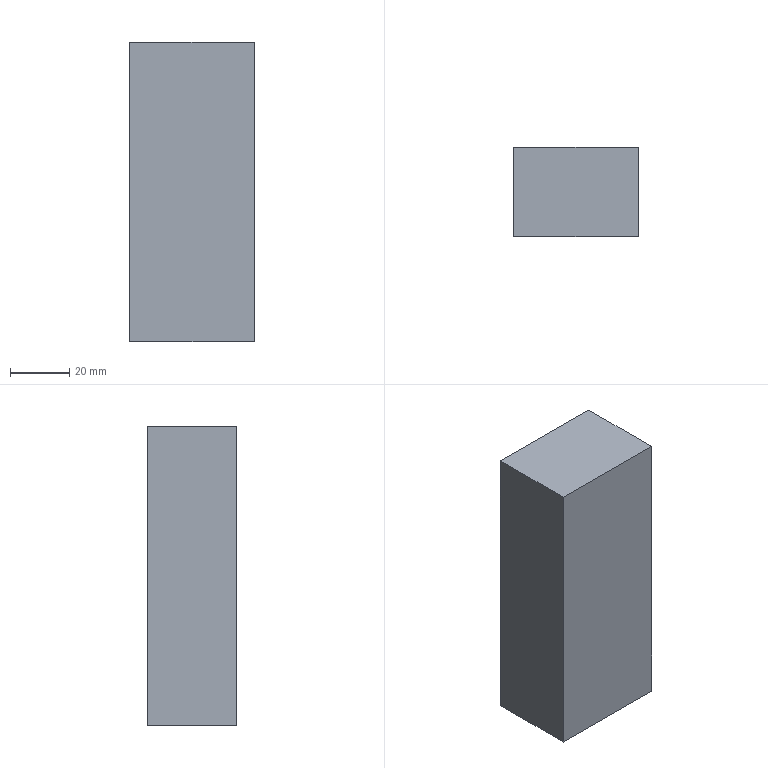Part | NX | features M5 螺纹孔1 2 | 1 solid | 6 faces | box 42 x 30 x 101 mm | volume 127260 mm3 | plane 6
STEP:
#1=CARTESIAN_POINT('',(-21.,201.666,187.866));
#2=VERTEX_POINT('',#1);
#3=CARTESIAN_POINT('',(-21.,201.666,86.866));
#4=VERTEX_POINT('',#3);
#5=CARTESIAN_POINT('',(-21.,201.666,116.575));
#6=DIRECTION('',(-0.000000012,0.,-1.));
#7=VECTOR('',#6,1000.);
#8=LINE('',#5,#7);
#9=EDGE_CURVE('',#2,#4,#8,.T.);
#10=ORIENTED_EDGE('',*,*,#9,.T.);
#11=CARTESIAN_POINT('',(-21.,171.666,86.866));
#12=VERTEX_POINT('',#11);
#13=CARTESIAN_POINT('',(-21.,137.875,86.866));
#14=DIRECTION('',(0.000000003,-1.,0.));
#15=VECTOR('',#14,1000.);
#16=LINE('',#13,#15);
#17=EDGE_CURVE('',#4,#12,#16,.T.);
#18=ORIENTED_EDGE('',*,*,#17,.T.);
#19=CARTESIAN_POINT('',(-21.,171.666,187.866));
#20=VERTEX_POINT('',#19);
#21=CARTESIAN_POINT('',(-21.,171.666,116.575));
#22=DIRECTION('',(-0.000000012,0.,-1.));
#23=VECTOR('',#22,1000.);
#24=LINE('',#21,#23);
#25=EDGE_CURVE('',#20,#12,#24,.T.);
#26=ORIENTED_EDGE('',*,*,#25,.F.);
#27=CARTESIAN_POINT('',(-21.,201.966,187.866));
#28=DIRECTION('',(0.000000003,-1.,0.));
#29=VECTOR('',#28,1000.);
#30=LINE('',#27,#29);
#31=EDGE_CURVE('',#2,#20,#30,.T.);
#32=ORIENTED_EDGE('',*,*,#31,.F.);
#33=EDGE_LOOP('',(#10,#18,#26,#32));
#34=FACE_BOUND('',#33,.T.);
#35=CARTESIAN_POINT('',(-21.,137.875,116.575));
#36=DIRECTION('',(1.,0.000000003,-0.000000012));
#37=DIRECTION('',(0.000000012,0.,1.));
#38=AXIS2_PLACEMENT_3D('',#35,#36,#37);
#39=PLANE('',#38);
#40=ADVANCED_FACE('',(#34),#39,.F.);
#41=CARTESIAN_POINT('',(21.,201.666,86.866));
#42=VERTEX_POINT('',#41);
#43=CARTESIAN_POINT('',(-25.,201.666,86.866));
#44=DIRECTION('',(1.,0.,-0.000000009));
#45=VECTOR('',#44,1000.);
#46=LINE('',#43,#45);
#47=EDGE_CURVE('',#4,#42,#46,.T.);
#48=ORIENTED_EDGE('',*,*,#47,.T.);
#49=CARTESIAN_POINT('',(21.,171.666,86.866));
#50=VERTEX_POINT('',#49);
#51=CARTESIAN_POINT('',(21.,130.666,86.866));
#52=DIRECTION('',(0.,-1.,0.));
#53=VECTOR('',#52,1000.);
#54=LINE('',#51,#53);
#55=EDGE_CURVE('',#42,#50,#54,.T.);
#56=ORIENTED_EDGE('',*,*,#55,.T.);
#57=CARTESIAN_POINT('',(-25.,171.666,86.866));
#58=DIRECTION('',(1.,0.,-0.000000009));
#59=VECTOR('',#58,1000.);
#60=LINE('',#57,#59);
#61=EDGE_CURVE('',#12,#50,#60,.T.);
#62=ORIENTED_EDGE('',*,*,#61,.F.);
#63=ORIENTED_EDGE('',*,*,#17,.F.);
#64=EDGE_LOOP('',(#48,#56,#62,#63));
#65=FACE_BOUND('',#64,.T.);
#66=CARTESIAN_POINT('',(-25.,130.666,86.866));
#67=DIRECTION('',(0.000000009,0.,1.));
#68=DIRECTION('',(0.,1.,0.));
#69=AXIS2_PLACEMENT_3D('',#66,#67,#68);
#70=PLANE('',#69);
#71=ADVANCED_FACE('',(#65),#70,.F.);
#72=CARTESIAN_POINT('',(21.,201.666,187.866));
#73=VERTEX_POINT('',#72);
#74=CARTESIAN_POINT('',(21.,201.666,126.866));
#75=DIRECTION('',(0.000000009,0.,1.));
#76=VECTOR('',#75,1000.);
#77=LINE('',#74,#76);
#78=EDGE_CURVE('',#42,#73,#77,.T.);
#79=ORIENTED_EDGE('',*,*,#78,.T.);
#80=CARTESIAN_POINT('',(21.,171.666,187.866));
#81=VERTEX_POINT('',#80);
#82=CARTESIAN_POINT('',(21.,176.666,187.866));
#83=DIRECTION('',(0.,-1.,0.));
#84=VECTOR('',#83,1000.);
#85=LINE('',#82,#84);
#86=EDGE_CURVE('',#73,#81,#85,.T.);
#87=ORIENTED_EDGE('',*,*,#86,.T.);
#88=CARTESIAN_POINT('',(21.,171.666,126.866));
#89=DIRECTION('',(0.000000009,0.,1.));
#90=VECTOR('',#89,1000.);
#91=LINE('',#88,#90);
#92=EDGE_CURVE('',#50,#81,#91,.T.);
#93=ORIENTED_EDGE('',*,*,#92,.F.);
#94=ORIENTED_EDGE('',*,*,#55,.F.);
#95=EDGE_LOOP('',(#79,#87,#93,#94));
#96=FACE_BOUND('',#95,.T.);
#97=CARTESIAN_POINT('',(21.,176.666,126.866));
#98=DIRECTION('',(-1.,0.,0.000000009));
#99=DIRECTION('',(-0.000000009,0.,-1.));
#100=AXIS2_PLACEMENT_3D('',#97,#98,#99);
#101=PLANE('',#100);
#102=ADVANCED_FACE('',(#96),#101,.F.);
#103=CARTESIAN_POINT('',(58.,201.666,187.866));
#104=DIRECTION('',(-1.,0.,0.000000019));
#105=VECTOR('',#104,1000.);
#106=LINE('',#103,#105);
#107=EDGE_CURVE('',#73,#2,#106,.T.);
#108=ORIENTED_EDGE('',*,*,#107,.T.);
#109=ORIENTED_EDGE('',*,*,#31,.T.);
#110=CARTESIAN_POINT('',(58.,171.666,187.866));
#111=DIRECTION('',(-1.,0.,0.000000019));
#112=VECTOR('',#111,1000.);
#113=LINE('',#110,#112);
#114=EDGE_CURVE('',#81,#20,#113,.T.);
#115=ORIENTED_EDGE('',*,*,#114,.F.);
#116=ORIENTED_EDGE('',*,*,#86,.F.);
#117=EDGE_LOOP('',(#108,#109,#115,#116));
#118=FACE_BOUND('',#117,.T.);
#119=CARTESIAN_POINT('',(58.,201.966,187.866));
#120=DIRECTION('',(-0.000000019,0.,-1.));
#121=DIRECTION('',(1.,0.,-0.000000019));
#122=AXIS2_PLACEMENT_3D('',#119,#120,#121);
#123=PLANE('',#122);
#124=ADVANCED_FACE('',(#118),#123,.F.);
#125=ORIENTED_EDGE('',*,*,#107,.F.);
#126=ORIENTED_EDGE('',*,*,#78,.F.);
#127=ORIENTED_EDGE('',*,*,#47,.F.);
#128=ORIENTED_EDGE('',*,*,#9,.F.);
#129=EDGE_LOOP('',(#125,#126,#127,#128));
#130=FACE_BOUND('',#129,.T.);
#131=CARTESIAN_POINT('',(-0.000001192,201.666,111.866));
#132=DIRECTION('',(0.,-1.,0.));
#133=DIRECTION('',(1.,0.,-0.000000009));
#134=AXIS2_PLACEMENT_3D('',#131,#132,#133);
#135=PLANE('',#134);
#136=ADVANCED_FACE('',(#130),#135,.F.);
#137=ORIENTED_EDGE('',*,*,#92,.T.);
#138=ORIENTED_EDGE('',*,*,#114,.T.);
#139=ORIENTED_EDGE('',*,*,#25,.T.);
#140=ORIENTED_EDGE('',*,*,#61,.T.);
#141=EDGE_LOOP('',(#137,#138,#139,#140));
#142=FACE_BOUND('',#141,.T.);
#143=CARTESIAN_POINT('',(-0.000001192,171.666,111.866));
#144=DIRECTION('',(0.,-1.,0.));
#145=DIRECTION('',(1.,0.,-0.000000009));
#146=AXIS2_PLACEMENT_3D('',#143,#144,#145);
#147=PLANE('',#146);
#148=ADVANCED_FACE('',(#142),#147,.T.);
#149=CLOSED_SHELL('',(#40,#71,#102,#124,#136,#148));
#150=MANIFOLD_SOLID_BREP('',#149);
#151=(LENGTH_UNIT()NAMED_UNIT(*)SI_UNIT(.MILLI.,.METRE.));
#152=UNCERTAINTY_MEASURE_WITH_UNIT(LENGTH_MEASURE(0.00001),#151,'','');
#153=(NAMED_UNIT(*)PLANE_ANGLE_UNIT()SI_UNIT($,.RADIAN.));
#154=(NAMED_UNIT(*)SI_UNIT($,.STERADIAN.)SOLID_ANGLE_UNIT());
#155=(GEOMETRIC_REPRESENTATION_CONTEXT(3)GLOBAL_UNCERTAINTY_ASSIGNED_CONTEXT((#152))GLOBAL_UNIT_ASSIGNED_CONTEXT((#151,#153,#154))REPRESENTATION_CONTEXT('',''));
#156=ADVANCED_BREP_SHAPE_REPRESENTATION('',(#150),#155);